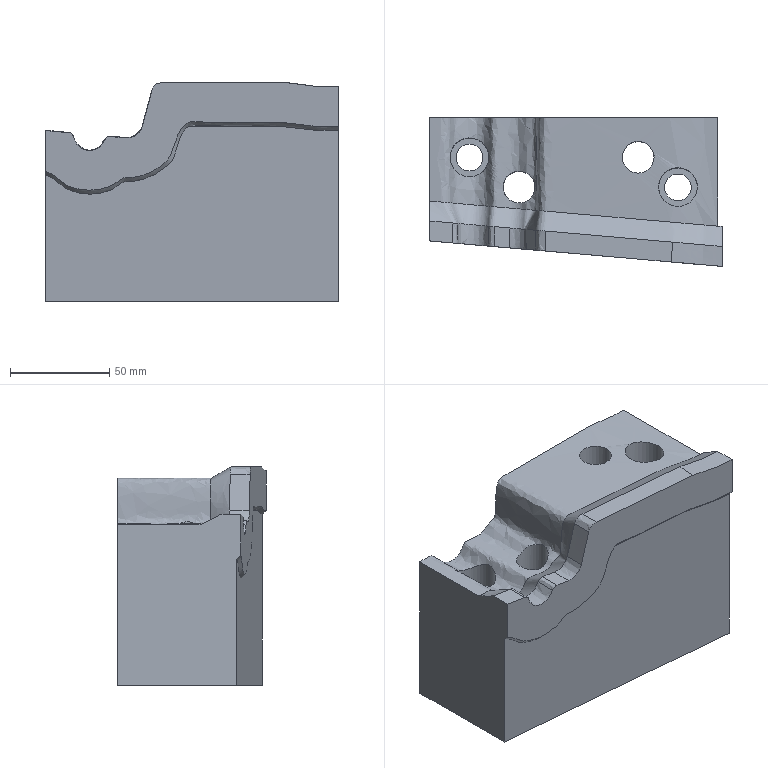Part | NX | features solid 2 | 1 solid | 29 faces | box 147.3 x 75 x 110.018 mm | volume 845941 mm3 | spline 13 | plane 10 | cylinder 6 | commonest cylinder face diameters 13.5 x2 16 x2 19.5 x2